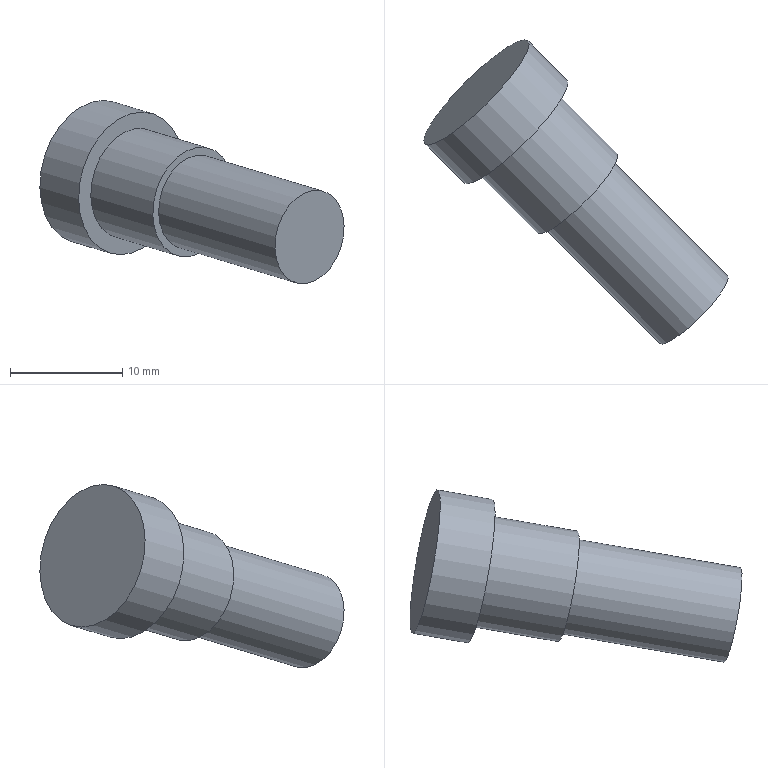Part | STEP file | gslz 2016.10.28-13_id1538_x_t | 1 solid | 7 faces | box 27.148 x 27.148 x 16.361 mm | volume 2153 mm3 | plane 4 | cylinder 3 | commonest cylinder face diameters 8.55 x1 10 x1 13 x1
STEP:
#1=CARTESIAN_POINT('',(0.,0.,0.));
#2=DIRECTION('',(0.,0.,1.));
#3=DIRECTION('',(1.,0.,0.));
#4=AXIS2_PLACEMENT_3D('',#1,#2,#3);
#5=CARTESIAN_POINT('',(1094.637,235.522,-12.036));
#6=VERTEX_POINT('',#5);
#7=CARTESIAN_POINT('',(1091.614,232.499,-12.036));
#8=DIRECTION('',(0.6917,-0.6917,-0.2079));
#9=DIRECTION('',(0.7071,0.7071,0.));
#10=AXIS2_PLACEMENT_3D('',#7,#8,#9);
#11=CIRCLE('',#10,4.275);
#12=CARTESIAN_POINT('',(1048.732,275.381,0.8542));
#13=DIRECTION('',(0.6917,-0.6917,-0.2079));
#14=DIRECTION('',(0.7071,0.7071,0.));
#15=AXIS2_PLACEMENT_3D('',#12,#13,#14);
#16=CYLINDRICAL_SURFACE('',#15,4.275);
#17=CARTESIAN_POINT('',(0.,62.));
#18=DIRECTION('',(1.,0.));
#19=VECTOR('',#18,1.);
#20=LINE('',#17,#19);
#21=(GEOMETRIC_REPRESENTATION_CONTEXT(2)PARAMETRIC_REPRESENTATION_CONTEXT()REPRESENTATION_CONTEXT('',''));
#22=DEFINITIONAL_REPRESENTATION('',(#20),#21);
#23=PCURVE('',#16,#22);
#24=CARTESIAN_POINT('',(1091.614,232.499,-12.036));
#25=DIRECTION('',(0.6917,-0.6917,-0.2079));
#26=DIRECTION('',(0.7071,0.7071,0.));
#27=AXIS2_PLACEMENT_3D('',#24,#25,#26);
#28=PLANE('',#27);
#29=CARTESIAN_POINT('',(0.,0.));
#30=DIRECTION('',(1.,0.));
#31=AXIS2_PLACEMENT_2D('',#29,#30);
#32=CIRCLE('',#31,4.275);
#33=(GEOMETRIC_REPRESENTATION_CONTEXT(2)PARAMETRIC_REPRESENTATION_CONTEXT()REPRESENTATION_CONTEXT('',''));
#34=DEFINITIONAL_REPRESENTATION('',(#32),#33);
#35=PCURVE('',#28,#34);
#36=SURFACE_CURVE('',#11,(#23,#35),.PCURVE_S1.);
#37=EDGE_CURVE('',#6,#6,#36,.T.);
#38=ORIENTED_EDGE('',*,*,#37,.T.);
#39=CARTESIAN_POINT('',(1105.012,225.147,-15.155));
#40=VERTEX_POINT('',#39);
#41=CARTESIAN_POINT('',(1094.637,235.522,-12.036));
#42=CARTESIAN_POINT('',(1105.012,225.147,-15.155));
#43=B_SPLINE_CURVE_WITH_KNOTS('',1,(#41,#42),.UNSPECIFIED.,.F.,.F.,(2,2),(62.,77.),.PIECEWISE_BEZIER_KNOTS.);
#44=CARTESIAN_POINT('',(6.283,0.));
#45=DIRECTION('',(0.,1.));
#46=VECTOR('',#45,1.);
#47=LINE('',#44,#46);
#48=(GEOMETRIC_REPRESENTATION_CONTEXT(2)PARAMETRIC_REPRESENTATION_CONTEXT()REPRESENTATION_CONTEXT('',''));
#49=DEFINITIONAL_REPRESENTATION('',(#47),#48);
#50=PCURVE('',#16,#49);
#51=CARTESIAN_POINT('',(0.,0.));
#52=DIRECTION('',(0.,1.));
#53=VECTOR('',#52,1.);
#54=LINE('',#51,#53);
#55=(GEOMETRIC_REPRESENTATION_CONTEXT(2)PARAMETRIC_REPRESENTATION_CONTEXT()REPRESENTATION_CONTEXT('',''));
#56=DEFINITIONAL_REPRESENTATION('',(#54),#55);
#57=PCURVE('',#16,#56);
#58=SEAM_CURVE('',#43,(#50,#57),.PCURVE_S1.);
#59=EDGE_CURVE('',#6,#40,#58,.T.);
#60=ORIENTED_EDGE('',*,*,#59,.T.);
#61=CARTESIAN_POINT('',(1098.966,219.101,-15.155));
#62=VERTEX_POINT('',#61);
#63=CARTESIAN_POINT('',(1101.989,222.124,-15.155));
#64=DIRECTION('',(-0.6917,0.6917,0.2079));
#65=DIRECTION('',(-0.7071,-0.7071,0.));
#66=AXIS2_PLACEMENT_3D('',#63,#64,#65);
#67=CIRCLE('',#66,4.275);
#68=CARTESIAN_POINT('',(9.425,77.));
#69=DIRECTION('',(-1.,0.));
#70=VECTOR('',#69,1.);
#71=LINE('',#68,#70);
#72=(GEOMETRIC_REPRESENTATION_CONTEXT(2)PARAMETRIC_REPRESENTATION_CONTEXT()REPRESENTATION_CONTEXT('',''));
#73=DEFINITIONAL_REPRESENTATION('',(#71),#72);
#74=PCURVE('',#16,#73);
#75=CARTESIAN_POINT('',(1101.989,222.124,-15.155));
#76=DIRECTION('',(-0.6917,0.6917,0.2079));
#77=DIRECTION('',(-0.7071,-0.7071,0.));
#78=AXIS2_PLACEMENT_3D('',#75,#76,#77);
#79=PLANE('',#78);
#80=CARTESIAN_POINT('',(0.,0.));
#81=DIRECTION('',(1.,0.));
#82=AXIS2_PLACEMENT_2D('',#80,#81);
#83=CIRCLE('',#82,4.275);
#84=(GEOMETRIC_REPRESENTATION_CONTEXT(2)PARAMETRIC_REPRESENTATION_CONTEXT()REPRESENTATION_CONTEXT('',''));
#85=DEFINITIONAL_REPRESENTATION('',(#83),#84);
#86=PCURVE('',#79,#85);
#87=SURFACE_CURVE('',#67,(#74,#86),.PCURVE_S1.);
#88=EDGE_CURVE('',#40,#62,#87,.T.);
#89=ORIENTED_EDGE('',*,*,#88,.T.);
#90=CARTESIAN_POINT('',(1101.989,222.124,-15.155));
#91=DIRECTION('',(-0.6917,0.6917,0.2079));
#92=DIRECTION('',(-0.7071,-0.7071,0.));
#93=AXIS2_PLACEMENT_3D('',#90,#91,#92);
#94=CIRCLE('',#93,4.275);
#95=CARTESIAN_POINT('',(3.142,77.));
#96=DIRECTION('',(-1.,0.));
#97=VECTOR('',#96,1.);
#98=LINE('',#95,#97);
#99=(GEOMETRIC_REPRESENTATION_CONTEXT(2)PARAMETRIC_REPRESENTATION_CONTEXT()REPRESENTATION_CONTEXT('',''));
#100=DEFINITIONAL_REPRESENTATION('',(#98),#99);
#101=PCURVE('',#16,#100);
#102=CARTESIAN_POINT('',(0.,0.));
#103=DIRECTION('',(1.,0.));
#104=AXIS2_PLACEMENT_2D('',#102,#103);
#105=CIRCLE('',#104,4.275);
#106=(GEOMETRIC_REPRESENTATION_CONTEXT(2)PARAMETRIC_REPRESENTATION_CONTEXT()REPRESENTATION_CONTEXT('',''));
#107=DEFINITIONAL_REPRESENTATION('',(#105),#106);
#108=PCURVE('',#79,#107);
#109=SURFACE_CURVE('',#94,(#101,#108),.PCURVE_S1.);
#110=EDGE_CURVE('',#62,#40,#109,.T.);
#111=ORIENTED_EDGE('',*,*,#110,.T.);
#112=ORIENTED_EDGE('',*,*,#59,.F.);
#113=EDGE_LOOP('',(#38,#60,#89,#111,#112));
#114=FACE_BOUND('',#113,.T.);
#115=ADVANCED_FACE('',(#114),#16,.T.);
#116=ORIENTED_EDGE('',*,*,#110,.F.);
#117=ORIENTED_EDGE('',*,*,#88,.F.);
#118=EDGE_LOOP('',(#116,#117));
#119=FACE_BOUND('',#118,.T.);
#120=ADVANCED_FACE('',(#119),#79,.F.);
#121=CARTESIAN_POINT('',(1095.15,236.034,-12.036));
#122=VERTEX_POINT('',#121);
#123=CARTESIAN_POINT('',(1091.614,232.499,-12.036));
#124=DIRECTION('',(0.6917,-0.6917,-0.2079));
#125=DIRECTION('',(0.7071,0.7071,0.));
#126=AXIS2_PLACEMENT_3D('',#123,#124,#125);
#127=CIRCLE('',#126,5.);
#128=CARTESIAN_POINT('',(0.,0.));
#129=DIRECTION('',(1.,0.));
#130=AXIS2_PLACEMENT_2D('',#128,#129);
#131=CIRCLE('',#130,5.);
#132=(GEOMETRIC_REPRESENTATION_CONTEXT(2)PARAMETRIC_REPRESENTATION_CONTEXT()REPRESENTATION_CONTEXT('',''));
#133=DEFINITIONAL_REPRESENTATION('',(#131),#132);
#134=PCURVE('',#28,#133);
#135=CARTESIAN_POINT('',(1091.614,232.499,-12.036));
#136=DIRECTION('',(-0.6917,0.6917,0.2079));
#137=DIRECTION('',(-0.7071,-0.7071,0.));
#138=AXIS2_PLACEMENT_3D('',#135,#136,#137);
#139=CYLINDRICAL_SURFACE('',#138,5.);
#140=CARTESIAN_POINT('',(9.425,0.));
#141=DIRECTION('',(-1.,0.));
#142=VECTOR('',#141,1.);
#143=LINE('',#140,#142);
#144=(GEOMETRIC_REPRESENTATION_CONTEXT(2)PARAMETRIC_REPRESENTATION_CONTEXT()REPRESENTATION_CONTEXT('',''));
#145=DEFINITIONAL_REPRESENTATION('',(#143),#144);
#146=PCURVE('',#139,#145);
#147=SURFACE_CURVE('',#127,(#134,#146),.PCURVE_S1.);
#148=EDGE_CURVE('',#122,#122,#147,.T.);
#149=ORIENTED_EDGE('',*,*,#148,.T.);
#150=EDGE_LOOP('',(#149));
#151=FACE_BOUND('',#150,.T.);
#152=ORIENTED_EDGE('',*,*,#37,.F.);
#153=EDGE_LOOP('',(#152));
#154=FACE_BOUND('',#153,.T.);
#155=ADVANCED_FACE('',(#151,#154),#28,.T.);
#156=CARTESIAN_POINT('',(1089.616,241.568,-10.373));
#157=VERTEX_POINT('',#156);
#158=CARTESIAN_POINT('',(1086.081,238.032,-10.373));
#159=DIRECTION('',(0.6917,-0.6917,-0.2079));
#160=DIRECTION('',(0.7071,0.7071,0.));
#161=AXIS2_PLACEMENT_3D('',#158,#159,#160);
#162=CIRCLE('',#161,5.);
#163=CARTESIAN_POINT('',(9.425,8.));
#164=DIRECTION('',(-1.,0.));
#165=VECTOR('',#164,1.);
#166=LINE('',#163,#165);
#167=(GEOMETRIC_REPRESENTATION_CONTEXT(2)PARAMETRIC_REPRESENTATION_CONTEXT()REPRESENTATION_CONTEXT('',''));
#168=DEFINITIONAL_REPRESENTATION('',(#166),#167);
#169=PCURVE('',#139,#168);
#170=CARTESIAN_POINT('',(1086.081,238.032,-10.373));
#171=DIRECTION('',(0.6917,-0.6917,-0.2079));
#172=DIRECTION('',(0.7071,0.7071,0.));
#173=AXIS2_PLACEMENT_3D('',#170,#171,#172);
#174=PLANE('',#173);
#175=CARTESIAN_POINT('',(0.,0.));
#176=DIRECTION('',(1.,0.));
#177=AXIS2_PLACEMENT_2D('',#175,#176);
#178=CIRCLE('',#177,5.);
#179=(GEOMETRIC_REPRESENTATION_CONTEXT(2)PARAMETRIC_REPRESENTATION_CONTEXT()REPRESENTATION_CONTEXT('',''));
#180=DEFINITIONAL_REPRESENTATION('',(#178),#179);
#181=PCURVE('',#174,#180);
#182=SURFACE_CURVE('',#162,(#169,#181),.PCURVE_S1.);
#183=EDGE_CURVE('',#157,#157,#182,.T.);
#184=ORIENTED_EDGE('',*,*,#183,.T.);
#185=CARTESIAN_POINT('',(1095.15,236.034,-12.036));
#186=CARTESIAN_POINT('',(1089.616,241.568,-10.373));
#187=B_SPLINE_CURVE_WITH_KNOTS('',1,(#185,#186),.UNSPECIFIED.,.F.,.F.,(2,2),(0.,8.),.PIECEWISE_BEZIER_KNOTS.);
#188=CARTESIAN_POINT('',(3.142,0.));
#189=DIRECTION('',(0.,1.));
#190=VECTOR('',#189,1.);
#191=LINE('',#188,#190);
#192=(GEOMETRIC_REPRESENTATION_CONTEXT(2)PARAMETRIC_REPRESENTATION_CONTEXT()REPRESENTATION_CONTEXT('',''));
#193=DEFINITIONAL_REPRESENTATION('',(#191),#192);
#194=PCURVE('',#139,#193);
#195=CARTESIAN_POINT('',(9.425,0.));
#196=DIRECTION('',(0.,1.));
#197=VECTOR('',#196,1.);
#198=LINE('',#195,#197);
#199=(GEOMETRIC_REPRESENTATION_CONTEXT(2)PARAMETRIC_REPRESENTATION_CONTEXT()REPRESENTATION_CONTEXT('',''));
#200=DEFINITIONAL_REPRESENTATION('',(#198),#199);
#201=PCURVE('',#139,#200);
#202=SEAM_CURVE('',#187,(#194,#201),.PCURVE_S1.);
#203=EDGE_CURVE('',#122,#157,#202,.T.);
#204=ORIENTED_EDGE('',*,*,#203,.F.);
#205=ORIENTED_EDGE('',*,*,#148,.F.);
#206=ORIENTED_EDGE('',*,*,#203,.T.);
#207=EDGE_LOOP('',(#184,#204,#205,#206));
#208=FACE_BOUND('',#207,.T.);
#209=ADVANCED_FACE('',(#208),#139,.T.);
#210=CARTESIAN_POINT('',(1090.677,242.628,-10.373));
#211=VERTEX_POINT('',#210);
#212=CARTESIAN_POINT('',(1086.081,238.032,-10.373));
#213=DIRECTION('',(0.6917,-0.6917,-0.2079));
#214=DIRECTION('',(0.7071,0.7071,0.));
#215=AXIS2_PLACEMENT_3D('',#212,#213,#214);
#216=CIRCLE('',#215,6.5);
#217=CARTESIAN_POINT('',(0.,0.));
#218=DIRECTION('',(1.,0.));
#219=AXIS2_PLACEMENT_2D('',#217,#218);
#220=CIRCLE('',#219,6.5);
#221=(GEOMETRIC_REPRESENTATION_CONTEXT(2)PARAMETRIC_REPRESENTATION_CONTEXT()REPRESENTATION_CONTEXT('',''));
#222=DEFINITIONAL_REPRESENTATION('',(#220),#221);
#223=PCURVE('',#174,#222);
#224=CARTESIAN_POINT('',(1084.698,239.415,-9.957));
#225=DIRECTION('',(-0.6917,0.6917,0.2079));
#226=DIRECTION('',(-0.7071,-0.7071,0.));
#227=AXIS2_PLACEMENT_3D('',#224,#225,#226);
#228=CYLINDRICAL_SURFACE('',#227,6.5);
#229=CARTESIAN_POINT('',(9.425,-2.));
#230=DIRECTION('',(-1.,0.));
#231=VECTOR('',#230,1.);
#232=LINE('',#229,#231);
#233=(GEOMETRIC_REPRESENTATION_CONTEXT(2)PARAMETRIC_REPRESENTATION_CONTEXT()REPRESENTATION_CONTEXT('',''));
#234=DEFINITIONAL_REPRESENTATION('',(#232),#233);
#235=PCURVE('',#228,#234);
#236=SURFACE_CURVE('',#216,(#223,#235),.PCURVE_S1.);
#237=EDGE_CURVE('',#211,#211,#236,.T.);
#238=ORIENTED_EDGE('',*,*,#237,.T.);
#239=EDGE_LOOP('',(#238));
#240=FACE_BOUND('',#239,.T.);
#241=ORIENTED_EDGE('',*,*,#183,.F.);
#242=EDGE_LOOP('',(#241));
#243=FACE_BOUND('',#242,.T.);
#244=ADVANCED_FACE('',(#240,#243),#174,.T.);
#245=ORIENTED_EDGE('',*,*,#237,.F.);
#246=CARTESIAN_POINT('',(1087.219,246.086,-9.333));
#247=VERTEX_POINT('',#246);
#248=CARTESIAN_POINT('',(1090.677,242.628,-10.373));
#249=CARTESIAN_POINT('',(1087.219,246.086,-9.333));
#250=B_SPLINE_CURVE_WITH_KNOTS('',1,(#248,#249),.UNSPECIFIED.,.F.,.F.,(2,2),(-2.,3.),.PIECEWISE_BEZIER_KNOTS.);
#251=CARTESIAN_POINT('',(9.425,0.));
#252=DIRECTION('',(0.,1.));
#253=VECTOR('',#252,1.);
#254=LINE('',#251,#253);
#255=(GEOMETRIC_REPRESENTATION_CONTEXT(2)PARAMETRIC_REPRESENTATION_CONTEXT()REPRESENTATION_CONTEXT('',''));
#256=DEFINITIONAL_REPRESENTATION('',(#254),#255);
#257=PCURVE('',#228,#256);
#258=CARTESIAN_POINT('',(3.142,0.));
#259=DIRECTION('',(0.,1.));
#260=VECTOR('',#259,1.);
#261=LINE('',#258,#260);
#262=(GEOMETRIC_REPRESENTATION_CONTEXT(2)PARAMETRIC_REPRESENTATION_CONTEXT()REPRESENTATION_CONTEXT('',''));
#263=DEFINITIONAL_REPRESENTATION('',(#261),#262);
#264=PCURVE('',#228,#263);
#265=SEAM_CURVE('',#250,(#257,#264),.PCURVE_S1.);
#266=EDGE_CURVE('',#211,#247,#265,.T.);
#267=ORIENTED_EDGE('',*,*,#266,.T.);
#268=CARTESIAN_POINT('',(1082.623,241.49,-9.333));
#269=DIRECTION('',(0.6917,-0.6917,-0.2079));
#270=DIRECTION('',(0.7071,0.7071,0.));
#271=AXIS2_PLACEMENT_3D('',#268,#269,#270);
#272=CIRCLE('',#271,6.5);
#273=CARTESIAN_POINT('',(9.425,3.));
#274=DIRECTION('',(-1.,0.));
#275=VECTOR('',#274,1.);
#276=LINE('',#273,#275);
#277=(GEOMETRIC_REPRESENTATION_CONTEXT(2)PARAMETRIC_REPRESENTATION_CONTEXT()REPRESENTATION_CONTEXT('',''));
#278=DEFINITIONAL_REPRESENTATION('',(#276),#277);
#279=PCURVE('',#228,#278);
#280=CARTESIAN_POINT('',(1082.623,241.49,-9.333));
#281=DIRECTION('',(-0.6917,0.6917,0.2079));
#282=DIRECTION('',(-0.7071,-0.7071,0.));
#283=AXIS2_PLACEMENT_3D('',#280,#281,#282);
#284=PLANE('',#283);
#285=CARTESIAN_POINT('',(-6.5,0.));
#286=CARTESIAN_POINT('',(-6.5,11.258));
#287=CARTESIAN_POINT('',(3.25,5.629));
#288=CARTESIAN_POINT('',(13.,0.));
#289=CARTESIAN_POINT('',(3.25,-5.629));
#290=CARTESIAN_POINT('',(-6.5,-11.258));
#291=CARTESIAN_POINT('',(-6.5,0.));
#292=(BOUNDED_CURVE()B_SPLINE_CURVE(2,(#285,#286,#287,#288,#289,#290,#291),.UNSPECIFIED.,.T.,.F.)B_SPLINE_CURVE_WITH_KNOTS((1,2,2,2,2,1),(-2.094,0.,2.094,4.189,6.283,8.378),.UNSPECIFIED.)CURVE()GEOMETRIC_REPRESENTATION_ITEM()RATIONAL_B_SPLINE_CURVE((1.,0.5,1.,0.5,1.,0.5,1.))REPRESENTATION_ITEM(''));
#293=(GEOMETRIC_REPRESENTATION_CONTEXT(2)PARAMETRIC_REPRESENTATION_CONTEXT()REPRESENTATION_CONTEXT('',''));
#294=DEFINITIONAL_REPRESENTATION('',(#292),#293);
#295=PCURVE('',#284,#294);
#296=SURFACE_CURVE('',#272,(#279,#295),.PCURVE_S1.);
#297=EDGE_CURVE('',#247,#247,#296,.T.);
#298=ORIENTED_EDGE('',*,*,#297,.T.);
#299=ORIENTED_EDGE('',*,*,#266,.F.);
#300=EDGE_LOOP('',(#245,#267,#298,#299));
#301=FACE_BOUND('',#300,.T.);
#302=ADVANCED_FACE('',(#301),#228,.T.);
#303=ORIENTED_EDGE('',*,*,#297,.F.);
#304=EDGE_LOOP('',(#303));
#305=FACE_BOUND('',#304,.T.);
#306=ADVANCED_FACE('',(#305),#284,.T.);
#307=CLOSED_SHELL('',(#115,#120,#155,#209,#244,#302,#306));
#308=MANIFOLD_SOLID_BREP('',#307);
#309=(LENGTH_UNIT()NAMED_UNIT(*)SI_UNIT(.MILLI.,.METRE.));
#310=UNCERTAINTY_MEASURE_WITH_UNIT(LENGTH_MEASURE(0.000005),#309,'','');
#311=(NAMED_UNIT(*)PLANE_ANGLE_UNIT()SI_UNIT($,.RADIAN.));
#312=(NAMED_UNIT(*)SI_UNIT($,.STERADIAN.)SOLID_ANGLE_UNIT());
#313=(GEOMETRIC_REPRESENTATION_CONTEXT(3)GLOBAL_UNCERTAINTY_ASSIGNED_CONTEXT((#310))GLOBAL_UNIT_ASSIGNED_CONTEXT((#309,#311,#312))REPRESENTATION_CONTEXT('',''));
#314=ADVANCED_BREP_SHAPE_REPRESENTATION('',(#4,#308),#313);